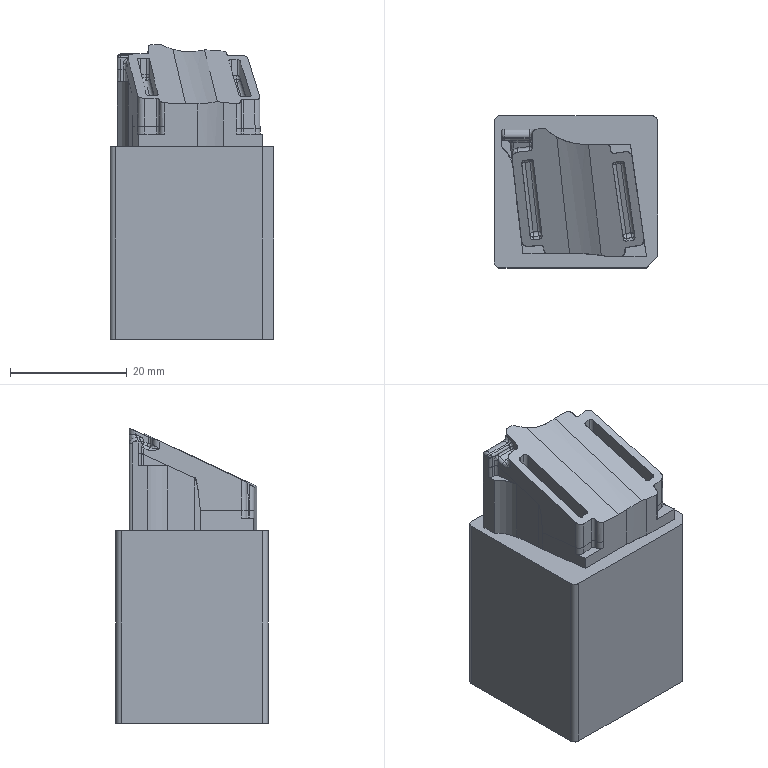NC program | NX | posted with a generic post | part box 28 x 26 x 50.455 mm
Whole program:
N10 G17 G21 G94 G90
(ZLEVEL_PROFILE_1 , TOOL : D0.8R0.4)
N12 T00 M6
N14 G54
N16 G17 G0 G90 X-6.275 Y10.043 S0 M3
N18 G43 Z10. H0
N20 Z0.1
N22 G94 G1 Z-0.1 F250.
N24 G3 X-7.073 Y10.354 R1.
N26 G1 X-7.11 Y10.351
N28 X-7.132 Y10.35
N30 X-7.253 Y10.569
N32 X-7.242 Y10.578
N34 G2 X-6.489 Y10.955 R0.719
N36 G3 X-5.597 Y11.259 R1.
N38 G1 Z0.1
N40 G0 Z0.3
N42 X-5.697 Y11.421
N44 Z0.001
N46 G1 Z-0.199
N48 G2 X-6.508 Y11.052 R1.
N50 G3 X-7.148 Y10.848 R1.
N52 G1 X-7.302 Y10.731
N54 X-7.495 Y10.35
N56 X-7.49 Y10.256
N58 X-7.486 Y10.238
N60 X-7.379 Y10.117
N62 X-7.364 Y10.114
N64 X-7.277 Y10.115
N66 G2 X-6.534 Y9.799 R1.
N68 G1 Z0.001
N70 G0 Z0.2
N72 X-7.015 Y9.528
N74 Z-0.099
N76 G1 Z-0.299
N78 G3 X-7.44 Y9.881 R1.
N80 G1 X-7.561 Y9.934
N82 X-7.625 Y10.051
N84 X-7.61 Y10.132
N86 X-7.628 Y10.31
N88 G2 X-7.084 Y10.956 R1.027
N90 G1 X-6.985 Y11.005
N92 X-6.51 Y11.091
N94 G3 X-5.888 Y11.476 R1.
N96 G1 Z-0.099
N98 G0 Z0.101
N100 X-5.707 Y11.513
N102 Z-0.198
N104 G1 Z-0.398
N106 G2 X-6.511 Y11.116 R1.
N108 G3 X-7.449 Y10.718 R1.284
N110 G1 X-7.52 Y10.646
N112 G3 X-7.683 Y9.798 R0.874
N114 G1 X-7.682 Y9.797
N116 X-7.67 Y9.778
N118 G3 X-7.302 Y9.682 R0.354
N120 G2 X-8.087 Y9.753 R1.
N122 G1 Z-0.198
N124 G0 Z0.001
N126 X-6.969 Y9.104
N128 Z-0.298
N130 G1 Z-0.498
N132 G3 X-7.482 Y9.447 R1.
N134 G2 X-7.811 Y9.914 R0.454
N136 X-6.865 Y11.065 R1.205
N138 X-6.156 Y11.118 R2.368
N140 G3 X-5.277 Y11.518 R1.
N142 G1 Z-0.298
N144 G0 Z-0.098
N146 X-5.6
N148 Z-0.397
N150 G1 Z-0.597
N152 G2 X-6.156 Y11.118 R0.5
N154 G3 X-7.302 Y10.858 R1.699
N156 X-7.758 Y9.456 R1.131
N158 X-7.482 Y9.232 R0.375
N160 G2 X-6.904 Y8.896 R1.
N162 G1 Z-0.397
N164 G0 Z-0.198
N166 X-6.771 Y8.697
N168 Z-0.497
N170 G1 Z-0.697
N172 G3 X-7.482 Y9.017 R1.
N174 G2 X-7.739 Y9.201 R0.279
N176 X-7.043 Y11.005 R1.307
N178 X-6.156 Y11.118 R2.033
N180 G3 X-5.257 Y11.518 R1.
N182 G1 Z-0.497
N184 G0 Z-0.297
N186 X-5.414
N188 Z-0.596
N190 G1 Z-0.796
N192 G2 X-6.211 Y11.118 R1.
N194 G1 X-6.429 Y11.117
N196 G3 X-7.82 Y9.204 R1.425
N198 G1 X-7.739 Y8.986
N200 G3 X-7.482 Y8.802 R0.276
N202 G2 X-6.764 Y8.483 R1.
N204 G1 Z-0.596
N206 G0 Z-0.397
N208 X-6.756 Y8.269
N210 Z-0.696
N212 G1 Z-0.896
N214 G3 X-7.483 Y8.587 R1.
N216 G2 X-7.739 Y8.77 R0.272
N218 X-7.901 Y9.533 R1.833
N220 G1 Y9.72
N222 G2 X-6.552 Y11.108 R1.387
N224 G1 X-6.211 Y11.118
N226 G3 X-5.437 Y11.518 R1.
N228 G1 Z-0.696
N230 G0 Z-0.496
N232 Z-0.795
N234 G1 Z-0.995
N236 G2 X-6.211 Y11.118 R1.
N238 G1 X-6.553 Y11.108
N240 G3 X-7.902 Y9.721 R1.386
N242 G1 X-7.901 Y9.318
N244 X-7.84 Y8.822
N246 X-7.727 Y8.534
N248 G3 X-7.483 Y8.372 R0.257
N250 G2 X-6.735 Y8.056 R1.
N252 G1 Z-0.795
N254 G0 Z-0.596
N256 X-6.736 Y7.841
N258 Z-0.895
N260 G1 Z-1.095
N262 G3 X-7.483 Y8.157 R1.
N264 G2 X-7.739 Y8.34 R0.264
N266 X-7.902 Y9.103 R1.879
N268 G1 Y9.722
N270 G2 X-6.553 Y11.108 R1.386
N272 G1 X-6.211 Y11.118
N274 G3 X-5.437 Y11.518 R1.
N276 G1 Z-0.895
N278 G0 Z-0.695
N280 X-5.287
N282 Z-0.995
N284 G1 Z-1.195
N286 G2 X-6.211 Y11.118 R1.
N288 G3 X-7.383 Y10.804 R1.638
N290 G1 X-7.421 Y10.774
N292 G3 X-7.903 Y9.716 R1.433
N294 G1 X-7.902 Y8.888
N296 G3 X-7.788 Y8.213 R2.639
N298 X-7.484 Y7.943 R0.391
N300 G2 X-6.9 Y7.608 R1.
N302 G1 Z-0.995
N304 G0 Z-0.795
N306 X-6.848 Y7.399
N308 Z-1.094
N310 G1 Z-1.294
N312 G3 X-7.484 Y7.728 R1.
N314 G2 X-7.739 Y7.909 R0.322
N316 X-7.902 Y8.673 R1.937
N318 G1 X-7.903 Y9.716
N320 G2 X-7.421 Y10.774 R1.411
N322 G1 X-7.334 Y10.843
N324 G2 X-6.211 Y11.118 R1.759
N326 G3 X-5.312 Y11.518 R1.
N328 G1 Z-1.094
N330 G0 Z0.3
N332 X-8.181 Y10.385
N334 Z-1.194
N336 G1 Z-1.394
N338 G2 X-7.904 Y9.695 R1.
N340 G1 X-7.903 Y8.458
N342 G3 X-7.739 Y7.694 R1.847
N344 X-7.484 Y7.513 R0.316
N346 G2 X-6.839 Y7.185 R1.
N348 G1 Z-1.194
N350 G0 Z-0.994
N352 X-7.427 Y6.902
N354 Z-1.293
N356 G1 Z-1.493
N358 G3 X-7.619 Y7.337 R1.
N360 G2 X-7.903 Y8.243 R1.375
N362 G1 X-7.904 Y9.356
N364 X-7.917 Y9.53
N366 G3 X-8.258 Y10.212 R1.
N368 G1 Z-1.293
N370 G0 Z-1.094
N372 X-7.903 Y8.362
N374 Z-1.293
N376 G1 Y7.76 Z-1.298
N378 X-7.835 Y7.529 Z-1.301
N380 X-7.903 Y7.76 Z-1.303
N382 X-7.904 Y9.147 Z-1.315
N384 X-7.914 Y9.282 Z-1.316
N386 X-7.904 Y9.147 Z-1.317
N388 X-7.903 Y7.76 Z-1.329
N390 X-7.835 Y7.529 Z-1.331
N392 X-7.903 Y7.76 Z-1.333
N394 X-7.904 Y9.147 Z-1.345
N396 X-7.914 Y9.282 Z-1.347
N398 X-7.904 Y9.147 Z-1.348
N400 X-7.903 Y7.76 Z-1.36
N402 X-7.835 Y7.529 Z-1.362
N404 X-7.903 Y7.76 Z-1.364
N406 X-7.904 Y9.147 Z-1.376
N408 X-7.914 Y9.282 Z-1.377
N410 X-7.904 Y9.147 Z-1.379
N412 X-7.903 Y7.76 Z-1.391
N414 X-7.835 Y7.529 Z-1.393
N416 X-7.903 Y7.76 Z-1.395
N418 X-7.904 Y9.147 Z-1.407
N420 X-7.914 Y9.282 Z-1.408
N422 X-7.904 Y9.147 Z-1.409
N424 X-7.903 Y7.76 Z-1.421
N426 X-7.835 Y7.529 Z-1.424
N428 X-7.903 Y7.76 Z-1.426
N430 X-7.904 Y9.147 Z-1.438
N432 X-7.914 Y9.282 Z-1.439
N434 X-7.904 Y9.147 Z-1.44
N436 X-7.903 Y7.76 Z-1.452
N438 X-7.835 Y7.529 Z-1.454
N440 X-7.903 Y7.76 Z-1.456
N442 X-7.904 Y9.147 Z-1.469
N444 X-7.914 Y9.282 Z-1.47
N446 X-7.904 Y9.147 Z-1.471
N448 X-7.903 Y7.76 Z-1.483
N450 X-7.835 Y7.529 Z-1.485
N452 X-7.903 Y7.76 Z-1.487
N454 X-7.904 Y9.147 Z-1.499
N456 X-7.914 Y9.282 Z-1.5
N458 X-7.904 Y9.147 Z-1.502
N460 X-7.903 Y7.76 Z-1.514
N462 X-7.835 Y7.529 Z-1.516
N464 X-7.903 Y7.76 Z-1.518
N466 X-7.904 Y9.147 Z-1.53
N468 X-7.914 Y9.282 Z-1.531
N470 X-7.904 Y9.147 Z-1.532
N472 X-7.903 Y7.76 Z-1.544
N474 X-7.835 Y7.529 Z-1.547
N476 X-7.903 Y7.76 Z-1.549
N478 X-7.904 Y9.147 Z-1.561
N480 X-7.914 Y9.282 Z-1.562
N482 X-7.904 Y9.147 Z-1.563
N484 X-7.903 Y7.76 Z-1.575
N486 X-7.835 Y7.529 Z-1.577
N488 X-7.903 Y7.76 Z-1.579
N490 X-7.904 Y9.147 Z-1.592
N492 X-7.914 Y9.282 Z-1.593
N494 X-7.904 Y9.147
N496 X-7.903 Y7.974
N498 G3 X-7.842 Y7.554 R1.493
N500 G1 X-7.739 Y7.201
N502 G3 X-7.58 Y7.072 R0.155
N504 G2 X-6.815 Y6.758 R1.
N506 G1 Z-1.393
N508 G0 Z-1.193
N510 X-10.936 Y6.445
N512 Z-1.492
N514 G1 Z-1.692
N516 G3 X-10.421 Y6.713 R1.
N518 G1 X-10.312 Y6.819
N520 X-7.981 Y7.16
N522 G3 X-7.852 Y7.326 R0.152
N524 G1 X-7.903 Y7.814
N526 X-7.905 Y8.927
N528 X-7.918 Y9.083
N530 G3 X-8.513 Y8.886 R1.
N532 G1 Z-1.492
N534 G0 Z-1.293
N536 X-8.453 Y8.688
N538 Z-1.492
N540 G2 X-8.453 Y8.688 Z-1.508 I0.268 J0.08
N542 X-8.453 Y8.688 Z-1.523 I0.268 J0.08
N544 X-8.453 Y8.688 Z-1.538 I0.268 J0.08
N546 X-8.453 Y8.688 Z-1.554 I0.268 J0.08
N548 X-8.453 Y8.688 Z-1.569 I0.268 J0.08
N550 X-8.453 Y8.688 Z-1.584 I0.268 J0.08
N552 X-8.453 Y8.688 Z-1.6 I0.268 J0.08
N554 X-8.453 Y8.688 Z-1.615 I0.268 J0.08
N556 X-8.453 Y8.688 Z-1.63 I0.268 J0.08
N558 X-8.453 Y8.688 Z-1.646 I0.268 J0.08
N560 X-8.453 Y8.688 Z-1.661 I0.268 J0.08
N562 X-8.453 Y8.688 Z-1.676 I0.268 J0.08
N564 X-8.453 Y8.688 Z-1.692 I0.268 J0.08
N566 X-8.453 Y8.688 Z-1.707 I0.268 J0.08
N568 X-8.453 Y8.688 Z-1.723 I0.268 J0.08
N570 X-8.453 Y8.688 Z-1.738 I0.268 J0.08
N572 X-8.453 Y8.688 Z-1.753 I0.268 J0.08
N574 X-8.453 Y8.688 Z-1.769 I0.268 J0.08
N576 X-8.453 Y8.688 Z-1.784 I0.268 J0.08
N578 X-7.912 Y8.831 Z-1.792 R-0.28
N580 G1 X-7.905 Y8.8
N582 X-7.903 Y7.342
N584 X-7.957 Y7.305
N586 X-10.12 Y7.032
N588 G3 X-10.78 Y6.527 R0.825
N590 G2 X-11.019 Y6.178 R1.
N592 G1 Z-1.592
N594 G0 Z-1.392
N596 X-10.954 Y5.691
N598 Z-1.691
N600 G1 Z-1.891
N602 G3 X-10.956 Y6.165 R1.
N604 G1 X-10.981 Y6.263
N606 X-10.983 Y6.284
N608 X-10.982 Y6.285
N610 G2 X-10.14 Y7.089 R1.027
N612 G3 X-8.015 Y7.348 R210.577
N614 G1 X-7.941 Y7.345
N616 X-7.892 Y7.401
N618 X-7.904 Y7.474
N620 X-7.905 Y8.56
N622 X-7.911 Y8.637
N624 G3 X-8.511 Y8.437 R1.
N626 G1 Z-1.691
N628 G0 Z-1.492
N630 X-8.373 Y8.204
N632 Z-1.691
N634 G2 X-8.373 Y8.204 Z-1.707 I0.187 J0.208
N636 X-8.373 Y8.204 Z-1.722 I0.187 J0.208
N638 X-8.373 Y8.204 Z-1.737 I0.187 J0.208
N640 X-8.373 Y8.204 Z-1.753 I0.187 J0.208
N642 X-8.373 Y8.204 Z-1.768 I0.187 J0.208
N644 X-8.373 Y8.204 Z-1.783 I0.187 J0.208
N646 X-8.373 Y8.204 Z-1.799 I0.187 J0.208
N648 X-8.373 Y8.204 Z-1.814 I0.187 J0.208
N650 X-8.373 Y8.204 Z-1.83 I0.187 J0.208
N652 X-8.373 Y8.204 Z-1.845 I0.187 J0.208
N654 X-8.373 Y8.204 Z-1.86 I0.187 J0.208
N656 X-8.373 Y8.204 Z-1.876 I0.187 J0.208
N658 X-8.373 Y8.204 Z-1.891 I0.187 J0.208
N660 X-8.373 Y8.204 Z-1.906 I0.187 J0.208
N662 X-8.373 Y8.204 Z-1.922 I0.187 J0.208
N664 X-8.373 Y8.204 Z-1.937 I0.187 J0.208
N666 X-8.373 Y8.204 Z-1.952 I0.187 J0.208
N668 X-8.373 Y8.204 Z-1.968 I0.187 J0.208
N670 X-8.373 Y8.204 Z-1.983 I0.187 J0.208
N672 X-7.985 Y8.608 Z-1.991 R-0.28
N674 G1 X-7.906 Y8.527
N676 X-7.904 Y7.428
N678 X-7.981 Y7.387
N680 X-8.728 Y7.294
N682 X-10.14 Y7.123
N684 X-10.331 Y7.075
N686 G3 X-11.09 Y6.034 R0.988
N688 G2 X-11.169 Y5.557 R1.
N690 G1 Z-1.791
N692 G0 Z-1.591
N694 X-11.062 Y5.236
N696 Z-1.89
N698 G1 Z-2.09
N700 G3 X-11.122 Y5.747 R1.
N702 G2 X-10.989 Y6.639 R0.899
N704 X-10.075 Y7.143 R1.387
N706 G1 X-7.962 Y7.388
N708 X-7.905 Y7.464
N710 X-7.906 Y8.435
N712 G3 X-8.573 Y8.18 R1.
N714 G1 Z-1.89
N716 G0 Z-1.691
N718 X-8.369 Y8.023
N720 Z-1.89
N722 G2 X-8.369 Y8.023 Z-1.906 I0.182 J0.212
N724 X-8.369 Y8.023 Z-1.921 I0.182 J0.212
N726 X-8.369 Y8.023 Z-1.936 I0.182 J0.212
N728 X-8.369 Y8.023 Z-1.952 I0.182 J0.212
N730 X-8.369 Y8.023 Z-1.967 I0.182 J0.212
N732 X-8.369 Y8.023 Z-1.983 I0.182 J0.212
N734 X-8.369 Y8.023 Z-1.998 I0.182 J0.212
N736 X-8.369 Y8.023 Z-2.013 I0.182 J0.212
N738 X-8.369 Y8.023 Z-2.029 I0.182 J0.212
N740 X-8.369 Y8.023 Z-2.044 I0.182 J0.212
N742 X-8.369 Y8.023 Z-2.059 I0.182 J0.212
N744 X-8.369 Y8.023 Z-2.075 I0.182 J0.212
N746 X-8.369 Y8.023 Z-2.09 I0.182 J0.212
N748 X-8.369 Y8.023 Z-2.105 I0.182 J0.212
N750 X-8.369 Y8.023 Z-2.121 I0.182 J0.212
N752 X-8.369 Y8.023 Z-2.136 I0.182 J0.212
N754 X-8.369 Y8.023 Z-2.151 I0.182 J0.212
N756 X-8.369 Y8.023 Z-2.167 I0.182 J0.212
N758 X-8.369 Y8.023 Z-2.182 I0.182 J0.212
N760 X-7.991 Y8.435 Z-2.19 R-0.28
N762 G1 X-7.907 Y8.353
N764 X-7.906 Y7.458
N766 X-8.007 Y7.384
N768 X-10.076 Y7.143
N770 G3 X-11.227 Y6.202 R1.357
N772 X-11.104 Y5.498 R0.787
N774 G2 X-10.909 Y4.998 R1.
N776 G1 Z-1.99
N778 G0 Z-1.79
N780 X-11.155 Y4.851
N782 Z-2.09
N784 G1 Z-2.29
N786 G3 X-11.213 Y5.484 R1.
N788 G2 X-11.195 Y6.321 R0.988
N790 G1 X-11.146 Y6.42
N792 G2 X-10.077 Y7.143 R1.394
N794 G1 X-8.009 Y7.384
N796 X-7.906 Y7.459
N798 X-7.907 Y8.333
N800 G3 X-8.602 Y8.05 R1.
N802 G1 Z-2.09
N804 G0 Z-1.89
N806 X-8.289 Y7.844
N808 Z-2.09
N810 G2 X-8.289 Y7.844 Z-2.105 I0.101 J0.261
N812 X-8.289 Y7.844 Z-2.12 I0.101 J0.261
N814 X-8.289 Y7.844 Z-2.136 I0.101 J0.261
N816 X-8.289 Y7.844 Z-2.151 I0.101 J0.261
N818 X-8.289 Y7.844 Z-2.166 I0.101 J0.261
N820 X-8.289 Y7.844 Z-2.182 I0.101 J0.261
N822 X-8.289 Y7.844 Z-2.197 I0.101 J0.261
N824 X-8.289 Y7.844 Z-2.212 I0.101 J0.261
N826 X-8.289 Y7.844 Z-2.228 I0.101 J0.261
N828 X-8.289 Y7.844 Z-2.243 I0.101 J0.261
N830 X-8.289 Y7.844 Z-2.258 I0.101 J0.261
N832 X-8.289 Y7.844 Z-2.274 I0.101 J0.261
N834 X-8.289 Y7.844 Z-2.289 I0.101 J0.261
N836 X-8.289 Y7.844 Z-2.304 I0.101 J0.261
N838 X-8.289 Y7.844 Z-2.32 I0.101 J0.261
N840 X-8.289 Y7.844 Z-2.335 I0.101 J0.261
N842 X-8.289 Y7.844 Z-2.351 I0.101 J0.261
N844 X-8.289 Y7.844 Z-2.366 I0.101 J0.261
N846 X-8.289 Y7.844 Z-2.381 I0.101 J0.261
N848 X-8.069 Y8.359 Z-2.389 R-0.28
N850 G1 X-7.908 Y8.284
N852 X-7.907 Y7.459
N854 X-8.007 Y7.385
N856 X-10.089 Y7.143
N858 G3 X-10.876 Y6.764 R1.338
N860 G1 X-10.947 Y6.693
N862 G3 X-11.269 Y5.502 R1.229
N864 G2 X-11.338 Y4.801 R1.
N866 G1 Z-2.189
N868 G0 Z-1.99
N870 X-11.554 Y4.95
N872 Z-2.289
N874 G1 Z-2.489
N876 G3 X-11.32 Y5.656 R1.
N878 G2 X-10.079 Y7.144 R1.412
N880 G1 X-8.006 Y7.385
N882 X-7.934 Y7.387
N884 X-7.889 Y7.446
N886 X-7.907 Y7.516
N888 X-7.908 Y8.229
N890 G3 X-8.587 Y7.962 R1.
N892 G1 Z-2.289
N894 G0 Z-2.089
N896 X-8.273 Y7.785
N898 Z-2.289
N900 G2 X-8.273 Y7.785 Z-2.304 I0.085 J0.267
N902 X-8.273 Y7.785 Z-2.319 I0.085 J0.267
N904 X-8.273 Y7.785 Z-2.335 I0.085 J0.267
N906 X-8.273 Y7.785 Z-2.35 I0.085 J0.267
N908 X-8.273 Y7.785 Z-2.365 I0.085 J0.267
N910 X-8.273 Y7.785 Z-2.381 I0.085 J0.267
N912 X-8.273 Y7.785 Z-2.396 I0.085 J0.267
N914 X-8.273 Y7.785 Z-2.411 I0.085 J0.267
N916 X-8.273 Y7.785 Z-2.427 I0.085 J0.267
N918 X-8.273 Y7.785 Z-2.442 I0.085 J0.267
N920 X-8.273 Y7.785 Z-2.457 I0.085 J0.267
N922 X-8.273 Y7.785 Z-2.473 I0.085 J0.267
N924 X-8.273 Y7.785 Z-2.488 I0.085 J0.267
N926 X-8.273 Y7.785 Z-2.504 I0.085 J0.267
N928 X-8.273 Y7.785 Z-2.519 I0.085 J0.267
N930 X-8.273 Y7.785 Z-2.534 I0.085 J0.267
N932 X-8.273 Y7.785 Z-2.55 I0.085 J0.267
N934 X-8.273 Y7.785 Z-2.565 I0.085 J0.267
N936 X-8.273 Y7.785 Z-2.58 I0.085 J0.267
N938 X-8.086 Y8.312 Z-2.588 R-0.28
N940 G1 X-7.909 Y8.243
N942 X-7.908 Y7.516
N944 X-7.889 Y7.446
N946 X-7.933 Y7.388
N948 X-8.005 Y7.386
N950 X-10.08 Y7.145
N952 G3 X-11.321 Y5.57 R1.415
N954 G1 X-11.305 Y5.435
N956 X-11.282 Y5.289
N958 G2 X-11.437 Y4.582 R1.
N960 G1 Z-2.388
N962 G0 Z-2.189
N964 X-11.488 Y4.5
N966 Z-2.488
N968 G1 Z-2.688
N970 G3 X-11.282 Y5.241 R1.
N972 G1 X-11.304 Y5.419
N974 X-11.322 Y5.571
N976 G2 X-10.081 Y7.145 R1.415
N978 G1 X-8.004 Y7.387
N980 X-7.933 Y7.388
N982 X-7.889 Y7.447
N984 X-7.908 Y7.516
N986 X-7.909 Y8.068
N988 X-7.914 Y8.196
N990 G3 X-8.627 Y7.905 R1.
N992 G1 Z-2.488
N994 G0 Z-2.288
N996 X-8.462 Y7.862
N998 Z-2.488
N1000 G2 X-8.462 Y7.862 Z-2.503 I0.276 J0.042
N1002 X-8.462 Y7.862 Z-2.518 I0.276 J0.042
N1004 X-8.462 Y7.862 Z-2.534 I0.276 J0.042
N1006 X-8.462 Y7.862 Z-2.549 I0.276 J0.042
N1008 X-8.462 Y7.862 Z-2.564 I0.276 J0.042
N1010 X-8.462 Y7.862 Z-2.58 I0.276 J0.042
N1012 X-8.462 Y7.862 Z-2.595 I0.276 J0.042
N1014 X-8.462 Y7.862 Z-2.611 I0.276 J0.042
N1016 X-8.462 Y7.862 Z-2.626 I0.276 J0.042
N1018 X-8.462 Y7.862 Z-2.641 I0.276 J0.042
N1020 X-8.462 Y7.862 Z-2.657 I0.276 J0.042
N1022 X-8.462 Y7.862 Z-2.672 I0.276 J0.042
N1024 X-8.462 Y7.862 Z-2.687 I0.276 J0.042
N1026 X-8.462 Y7.862 Z-2.703 I0.276 J0.042
N1028 X-8.462 Y7.862 Z-2.718 I0.276 J0.042
N1030 X-8.462 Y7.862 Z-2.733 I0.276 J0.042
N1032 X-8.462 Y7.862 Z-2.749 I0.276 J0.042
N1034 X-8.462 Y7.862 Z-2.764 I0.276 J0.042
N1036 X-8.462 Y7.862 Z-2.779 I0.276 J0.042
N1038 X-7.909 Y7.951 Z-2.787 R-0.28
N1040 G1 Y7.515
N1042 X-7.893 Y7.444
N1044 X-7.939 Y7.386
N1046 X-8.012
N1048 X-10.082 Y7.145
N1050 G3 X-11.323 Y5.571 R1.415
N1052 G2 X-11.614 Y4.739 R1.
N1054 G1 Z-2.587
N1056 G0 Z-2.388
N1058 X-11.625 Y4.73
N1060 Z-2.687
N1062 G1 Z-2.887
N1064 G3 X-11.324 Y5.572 R1.
N1066 G2 X-10.083 Y7.146 R1.415
N1068 G1 X-7.976 Y7.391
N1070 X-7.902 Y7.419
N1072 X-7.909 Y7.499
N1074 Y7.638
N1076 X-7.911 Y7.73
N1078 G3 X-8.264 Y7.584 R0.5
N1080 G1 Z-2.687
N1082 G0 Z-2.487
N1084 X-9.246 Y7.244
N1086 Z-2.687
N1088 G1 X-9.58 Y7.205 Z-2.69
N1090 X-8.136 Y7.373 Z-2.702
N1092 X-7.999 Y7.392 Z-2.704
N1094 X-7.977 Y7.398
N1096 X-7.898 Y7.424 Z-2.705
N1098 X-7.894 Y7.431
N1100 X-7.911 Y7.512
N1102 X-7.894 Y7.431 Z-2.706
N1104 X-7.898 Y7.424
N1106 X-7.977 Y7.398 Z-2.707
N1108 X-7.999 Y7.392
N1110 X-8.136 Y7.373 Z-2.708
N1112 X-9.58 Y7.205 Z-2.721
N1114 X-8.136 Y7.373 Z-2.734
N1116 X-7.999 Y7.392 Z-2.735
N1118 X-7.977 Y7.398
N1120 X-7.898 Y7.424 Z-2.736
N1122 X-7.894 Y7.431
N1124 X-7.911 Y7.512 Z-2.737
N1126 X-7.894 Y7.431
N1128 X-7.898 Y7.424
N1130 X-7.977 Y7.398 Z-2.738
N1132 X-7.999 Y7.392
N1134 X-8.136 Y7.373 Z-2.739
N1136 X-9.58 Y7.205 Z-2.752
N1138 X-8.136 Y7.373 Z-2.765
N1140 X-7.999 Y7.392 Z-2.766
N1142 X-7.977 Y7.398
N1144 X-7.898 Y7.424 Z-2.767
N1146 X-7.894 Y7.431
N1148 X-7.911 Y7.512 Z-2.768
N1150 X-7.894 Y7.431 Z-2.769
N1152 X-7.898 Y7.424
N1154 X-7.977 Y7.398
N1156 X-7.999 Y7.392
N1158 X-8.136 Y7.373 Z-2.771
N1160 X-9.58 Y7.205 Z-2.783
N1162 X-8.136 Y7.373 Z-2.796
N1164 X-7.999 Y7.392 Z-2.797
N1166 X-7.977 Y7.398
N1168 X-7.898 Y7.424 Z-2.798
N1170 X-7.894 Y7.431
N1172 X-7.911 Y7.512 Z-2.799
N1174 X-7.894 Y7.431 Z-2.8
N1176 X-7.898 Y7.424
N1178 X-7.977 Y7.398 Z-2.801
N1180 X-7.999 Y7.392
N1182 X-8.136 Y7.373 Z-2.802
N1184 X-9.58 Y7.205 Z-2.815
N1186 X-8.136 Y7.373 Z-2.827
N1188 X-7.999 Y7.392 Z-2.829
N1190 X-7.977 Y7.398
N1192 X-7.898 Y7.424
N1194 X-7.894 Y7.431 Z-2.83
N1196 X-7.911 Y7.512
N1198 X-7.894 Y7.431 Z-2.831
N1200 X-7.898 Y7.424
N1202 X-7.977 Y7.398 Z-2.832
N1204 X-7.999 Y7.392
N1206 X-8.136 Y7.373 Z-2.833
N1208 X-9.58 Y7.205 Z-2.846
N1210 X-8.136 Y7.373 Z-2.859
N1212 X-7.999 Y7.392 Z-2.86
N1214 X-7.977 Y7.398
N1216 X-7.898 Y7.424 Z-2.861
N1218 X-7.894 Y7.431
N1220 X-7.911 Y7.512
N1222 X-7.894 Y7.431 Z-2.862
N1224 X-7.898 Y7.424
N1226 X-7.977 Y7.398 Z-2.863
N1228 X-7.999 Y7.392
N1230 X-8.136 Y7.373 Z-2.864
N1232 X-9.58 Y7.205 Z-2.877
N1234 X-8.136 Y7.373 Z-2.89
N1236 X-7.999 Y7.392 Z-2.891
N1238 X-7.977 Y7.398
N1240 X-7.898 Y7.424 Z-2.892
N1242 X-7.894 Y7.431
N1244 X-7.911 Y7.512 Z-2.893
N1246 X-7.894 Y7.431
N1248 X-7.898 Y7.424
N1250 X-7.977 Y7.398 Z-2.894
N1252 X-7.999 Y7.392
N1254 X-8.136 Y7.373 Z-2.896
N1256 X-9.58 Y7.205 Z-2.908
N1258 X-8.136 Y7.373 Z-2.921
N1260 X-7.999 Y7.392 Z-2.922
N1262 X-7.977 Y7.398
N1264 X-7.898 Y7.424 Z-2.923
N1266 X-7.894 Y7.431
N1268 X-7.911 Y7.512 Z-2.924
N1270 X-7.894 Y7.431 Z-2.925
N1272 X-7.898 Y7.424
N1274 X-7.977 Y7.398
N1276 X-7.999 Y7.392 Z-2.926
N1278 X-8.136 Y7.373 Z-2.927
N1280 X-9.58 Y7.205 Z-2.94
N1282 X-8.136 Y7.373 Z-2.952
N1284 X-7.999 Y7.392 Z-2.953
N1286 X-7.977 Y7.398 Z-2.954
N1288 X-7.898 Y7.424
N1290 X-7.894 Y7.431
N1292 X-7.911 Y7.512 Z-2.955
N1294 X-7.894 Y7.431 Z-2.956
N1296 X-7.898 Y7.424
N1298 X-7.977 Y7.398 Z-2.957
N1300 X-7.999 Y7.392
N1302 X-8.136 Y7.373 Z-2.958
N1304 X-9.58 Y7.205 Z-2.971
N1306 X-8.136 Y7.373 Z-2.983
N1308 X-7.999 Y7.392 Z-2.985
N1310 X-7.977 Y7.398
N1312 X-7.898 Y7.424 Z-2.986
N1314 X-7.894 Y7.431
N1316 X-7.911 Y7.512
N1318 X-7.884 Y7.456
N1320 X-7.915 Y7.402
N1322 X-7.977 Y7.398
N1324 X-7.999 Y7.392
N1326 X-8.136 Y7.373
N1328 X-10.084 Y7.146
N1330 G3 X-11.325 Y5.572 R1.415
N1332 G2 X-11.627 Y4.73 R1.
N1334 G1 Z-2.786
N1336 G0 Z-2.587
N1338 Y4.726
N1340 Z-2.886
N1342 G1 Z-3.086
N1344 G3 X-11.326 Y5.572 R1.
N1346 G2 X-10.112 Y7.141 R1.406
N1348 G1 X-9.703 Y7.194
N1350 G3 X-9.371 Y7.385 R0.5
N1352 G1 Z-2.886
N1354 G0 Z-2.686
N1356 X-11.131 Y7.1
N1358 Z-2.985
N1360 G1 Z-3.185
N1362 X-10.352 Y7.279
N1364 G2 X-10.597 Y6.985 R0.5
N1366 G3 X-11.327 Y5.573 R1.386
N1368 G2 X-11.627 Y4.717 R1.
N1370 G1 Z-2.985
N1372 G0 Z-2.786
N1374 X-11.631 Y4.743
N1376 Z-3.085
N1378 G1 Z-3.285
N1380 G3 X-11.328 Y5.573 R1.
N1382 G2 X-10.884 Y6.783 R1.454
N1384 G3 X-10.728 Y7.133 R0.5
N1386 G1 X-11.237 Y6.995
N1388 Z-3.085
N1390 G0 Z-2.885
N1392 X-11.35 Y6.858
N1394 Z-3.185
N1396 G1 Z-3.385
N1398 X-10.978 Y6.951
N1400 G2 X-11.065 Y6.578 R0.5
N1402 G3 X-11.329 Y5.574 R1.461
N1404 G2 X-11.632 Y4.745 R1.
N1406 G1 Z-3.185
N1408 G0 Z10.
N1410 M5
N1412 M2